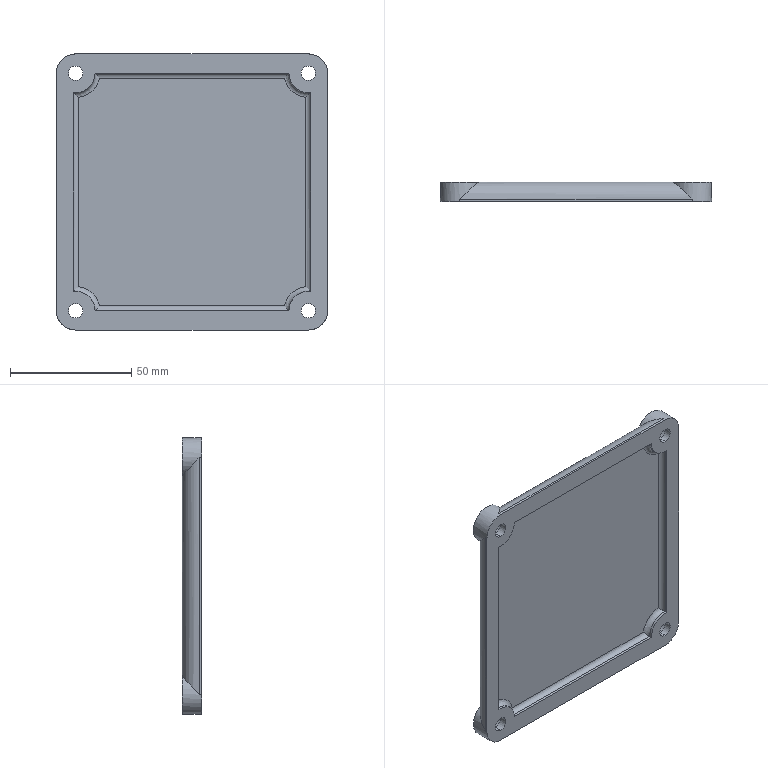Part | SolidWorks | features Fillet 2, ICE 2, Extrusion 1, HoleWzd 1 | 1 solid | 57 faces | box 112 x 8 x 114 mm | volume 68573 mm3 | cylinder 36 | plane 15 | torus 6 | commonest cylinder face diameters 16 x12 6 x8 9 x8 4 x4 14 x4